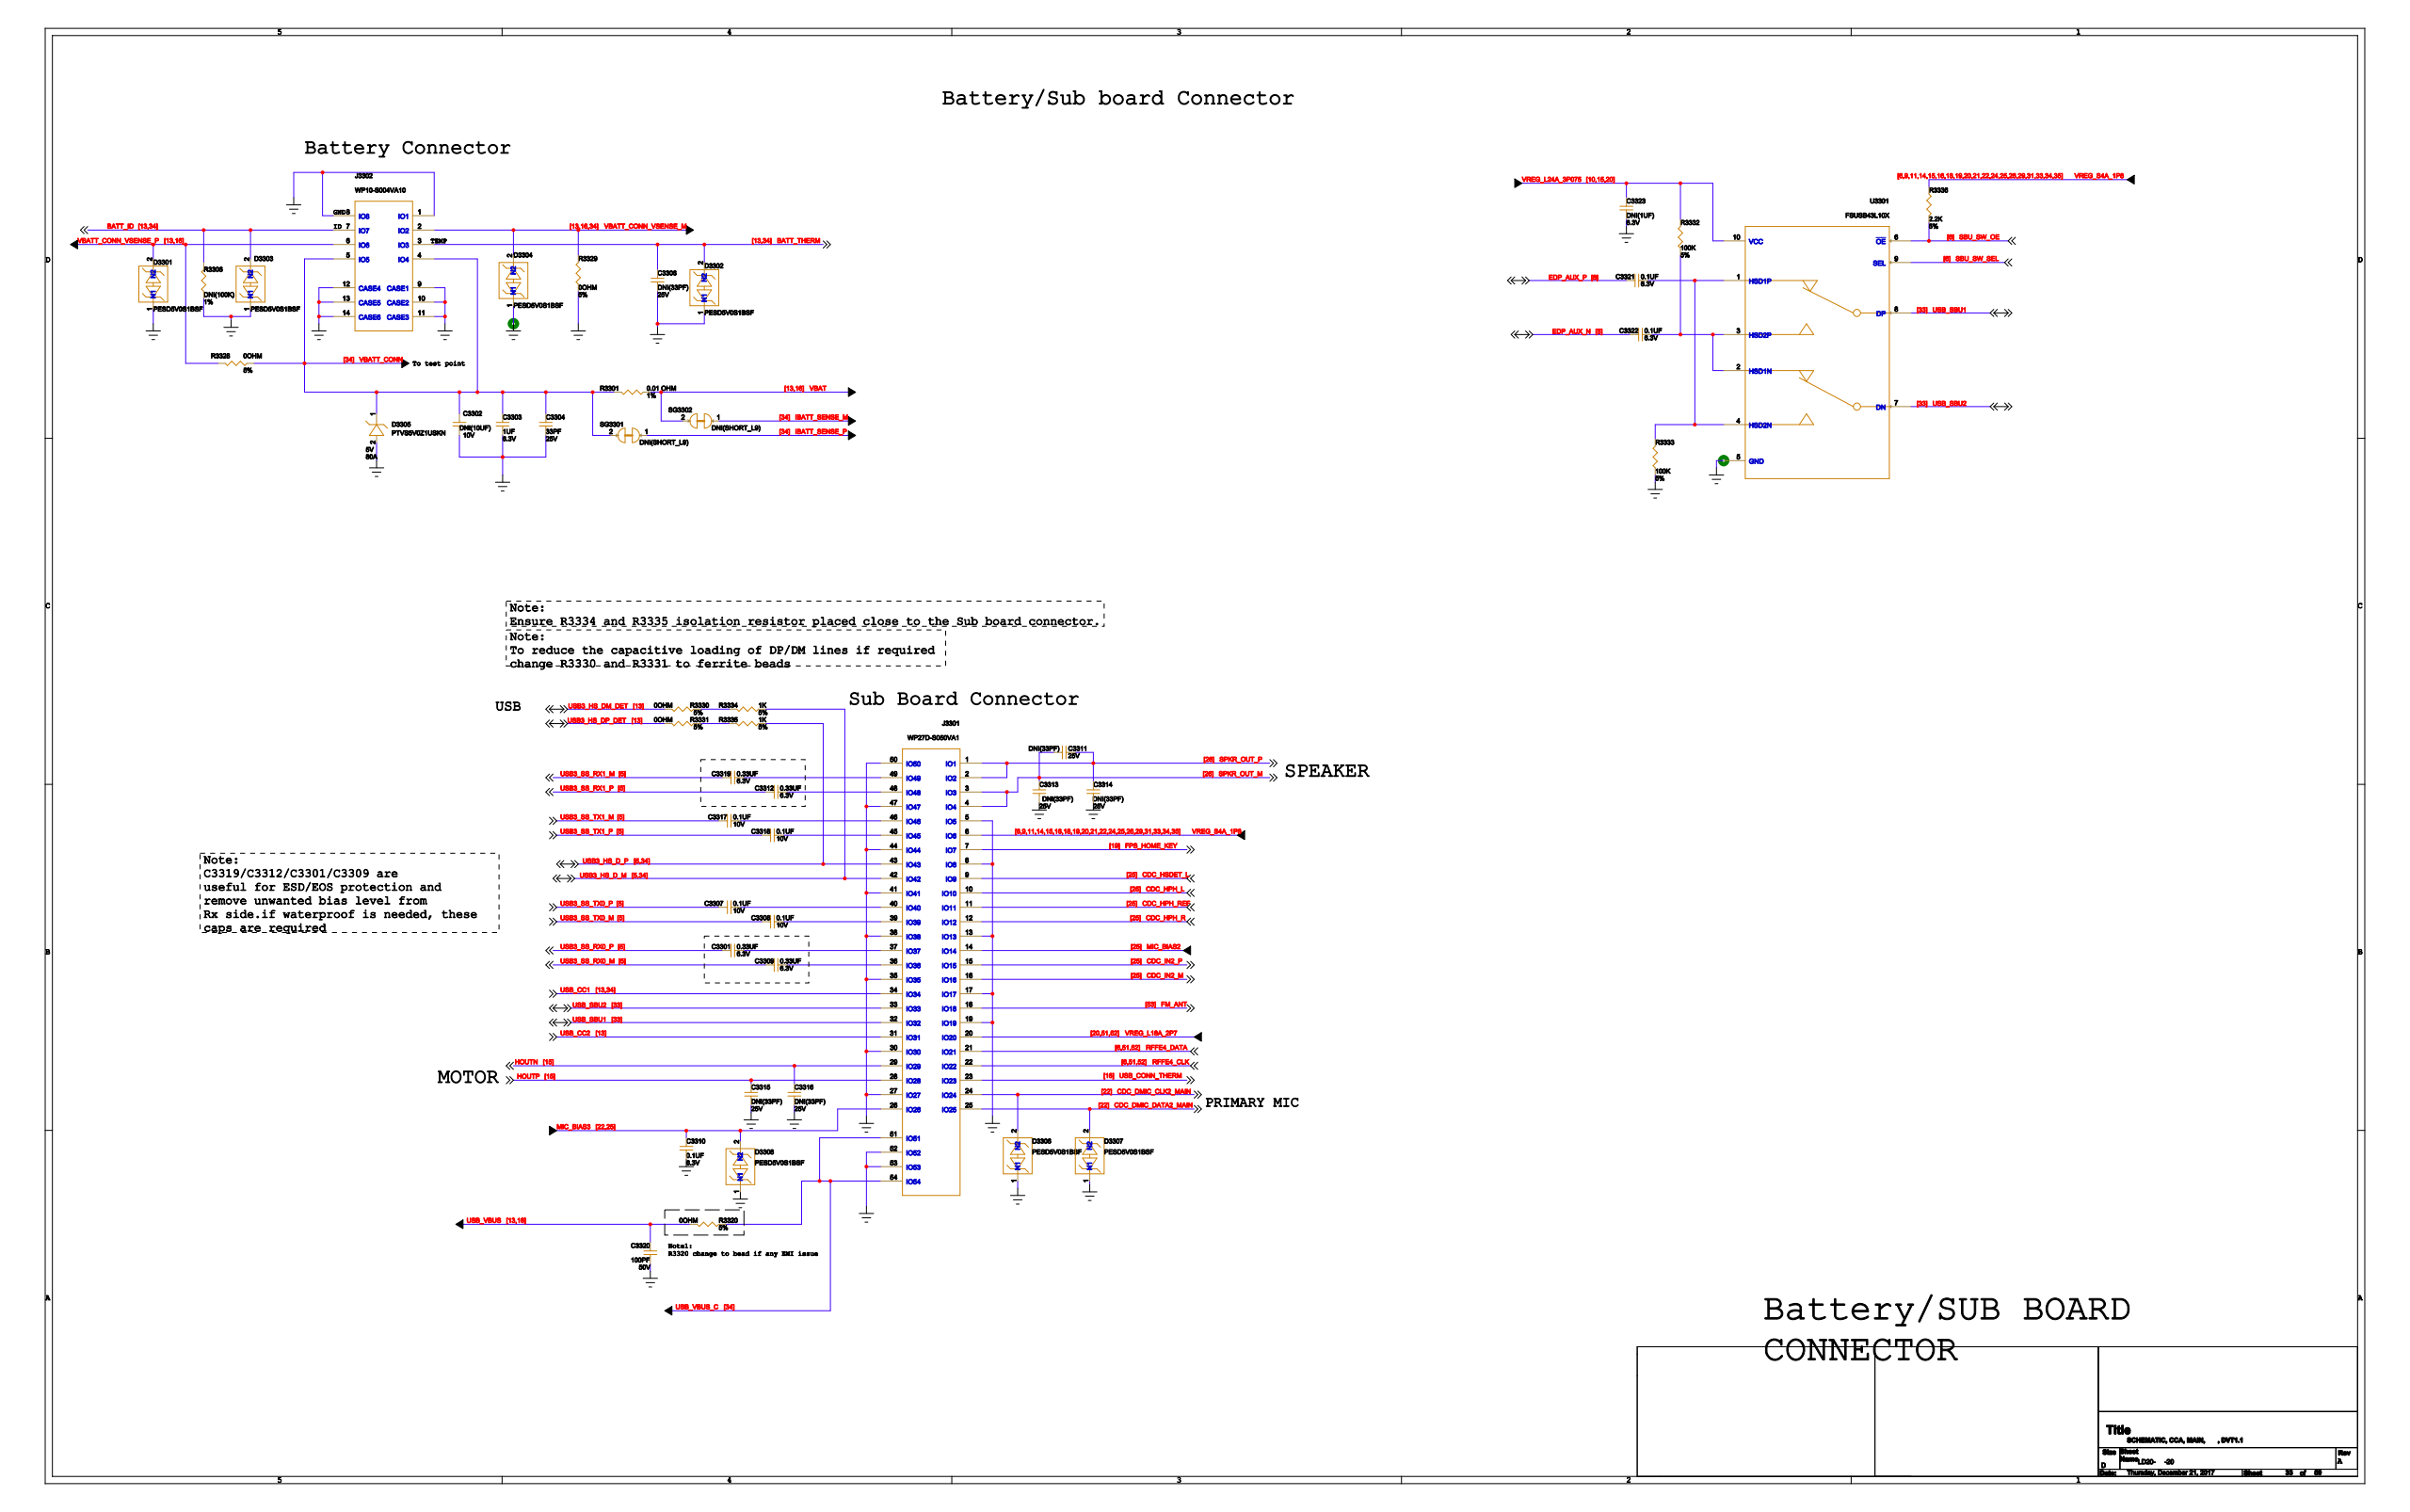Circuit board | Cadence Allegro | 1520 parts | 1149 nets | one sheet of the schematic
Parts on this sheet (reference | value | footprint):
C3301 | 0.33UF | 2P0201R
C3302 | DNI(10UF) | 2P0402RV1_DNI
C3303 | 1UF | 2P0201R
C3304 | 33PF | 2P0201R
C3306 | DNI(33PF) | 2P0201R_DNI
C3307 | 0.1UF | 2P0201R
C3308 | 0.1UF | 2P0201R
C3309 | 0.33UF | 2P0201R
C3310 | 0.1UF | 2P0201R
C3311 | DNI(33PF) | 2P0201R_DNI
C3312 | 0.33UF | 2P0201R
C3313 | DNI(33PF) | 2P0201R_DNI
C3314 | DNI(33PF) | 2P0201R_DNI
C3315 | DNI(33PF) | 2P0201R_DNI
C3316 | DNI(33PF) | 2P0201R_DNI
C3317 | 0.1UF | 2P0201R
C3318 | 0.1UF | 2P0201R
C3319 | 0.33UF | 2P0201R
C3320 | 100PF | 2P0201R
C3321 | 0.1UF | 2P0201R
C3322 | 0.1UF | 2P0201R
C3323 | DNI(1UF) | 2P0201R_DNI
D3301 | PESD5V0S1BSF | 2PSM25X13N
D3302 | PESD5V0S1BSF | 2PSM25X13N
D3303 | PESD5V0S1BSF | 2PSM25X13N
D3304 | PESD5V0S1BSF | 2PSM25X13N
D3305 | PTVS5V0Z1USKN | 2PSM68X31N
D3306 | PESD5V0S1BSF | 2PSM25X13N
D3307 | PESD5V0S1BSF | 2PSM25X13N
D3308 | PESD5V0S1BSF | 2PSM25X13N
J3301 | WP27D-S050VA1 | 54SCONS138V1_CCW
J3302 | WP10-S004VA10 | 14SCONS157V11-SH
R3301 | 0.01 OHM | 2P0805R
R3306 | DNI(100K) | 2P0201R_DNI
R3320 | 0OHM | 2P0805R
R3328 | 0OHM | 2P0201R
R3329 | 0OHM | 2P0201R
R3330 | 0OHM | 2P0402R
R3331 | 0OHM | 2P0402R
R3332 | 100K | 2P0201R
R3333 | 100K | 2P0201R
R3334 | 1K | 2P0201R
R3335 | 1K | 2P0201R
R3336 | 2.2K | 2P0201R
SG3301 | DNI(SHORT_L9) | SHORT_L9_2REC08X12
SG3302 | DNI(SHORT_L9) | SHORT_L9_2REC08X12
U3301 | FSUSB43L10X | 10PSM87X67N197
Nets of these parts (net: part-pin ...):
GND: C3302-2 C3303-2 C3304-2 C3306-2 C3310-2 C3313-2 C3314-2 C3315-2 C3316-2 C3320-2 C3323-2 D3301-1 D3302-1 D3303-1 D3304-1 D3305-2 D3306-1 D3307-1 D3308-1 J3302-1 J3302-8 J3302-9 J3302-10 J3302-11 J3302-12 J3302-13 J3302-14 R3306-2 R3329-2 R3333-2 U3301-5 J3301-5 J3301-8 J3301-13 J3301-17 J3301-19 J3301-27 J3301-30 J3301-35 J3301-38 J3301-41 J3301-44 J3301-47 J3301-50 J3301-52 J3301-53
VREG_S4A_1P8: R3336-2 J3301-6
MIC_BIAS3: C3310-1 D3308-2 J3301-26
IBATT_SENSE_P: SG3301-1
VBATT_CONN: C3302-1 C3303-1 C3304-1 D3305-1 J3302-4 J3302-5 R3301-1 R3328-2 SG3301-2
IBATT_SENSE_M: SG3302-1
VBAT: R3301-2 SG3302-2
VREG_L24A_3P075: C3323-1 R3332-1 U3301-10
USB3_SS_RX0_P: C3301-1
N35756340: C3301-2 J3301-37
USB3_SS_RX0_M: C3309-1
N35756342: C3309-2 J3301-36
USB3_SS_RX1_P: C3312-1
N35756432: C3312-2 J3301-48
USB3_SS_RX1_M: C3319-1
N35756416: C3319-2 J3301-49
USB_SBU2: U3301-7 J3301-33
USB_SBU1: U3301-8 J3301-32
N50099939: C3322-2 R3332-2 U3301-2 U3301-3
N50099935: C3321-2 R3333-1 U3301-1 U3301-4
SBU_SW_OE: R3336-1 U3301-6
SBU_SW_SEL: U3301-9
CDC_DMIC_CLK2_MAIN: D3306-2 J3301-24
CDC_DMIC_DATA2_MAIN: D3307-2 J3301-25
CDC_IN2_M: J3301-16
CDC_IN2_P: J3301-15
CDC_HPH_L: J3301-10
CDC_HPH_R: J3301-12
CDC_HPH_REF: J3301-11
CDC_HSDET_L: J3301-9
MIC_BIAS2: J3301-14
FM_ANT: J3301-18
VBATT_CONN_VSENSE_P: D3301-2 J3302-6 R3328-1
BATT_THERM: C3306-1 D3302-2 J3302-3
BATT_ID: D3303-2 J3302-7 R3306-1
VBATT_CONN_VSENSE_M: D3304-2 J3302-2 R3329-1
USB_CONN_THERM: J3301-23
USB_VBUS: C3320-1 R3320-2
HOUTP: C3315-1 J3301-28
HOUTN: C3316-1 J3301-29
EDP_AUX_P: C3321-1
EDP_AUX_N: C3322-1
USB3_SS_TX0_P: C3307-1
N35756510: C3307-2 J3301-40
USB3_SS_TX0_M: C3308-1
N35756506: C3308-2 J3301-39
USB3_SS_TX1_M: C3317-1
N35756582: C3317-2 J3301-46
USB3_SS_TX1_P: C3318-1
N35756584: C3318-2 J3301-45
VREG_L18A_2P7: J3301-20
SPKR_OUT_M: C3311-1 C3313-1 J3301-3 J3301-4
SPKR_OUT_P: C3311-2 C3314-1 J3301-1 J3301-2
USB_CC2: J3301-31
USB_CC1: J3301-34
RFFE4_CLK: J3301-22
RFFE4_DATA: J3301-21
USB3_HS_D_M: R3334-2 J3301-42
USB3_HS_D_P: R3335-2 J3301-43
USB_VBUS_C: R3320-1 J3301-51 J3301-54
FPS_HOME_KEY: J3301-7
N50098624: R3330-1 R3334-1
USB3_HS_DM_DET: R3330-2
N50098630: R3331-1 R3335-1
USB3_HS_DP_DET: R3331-2